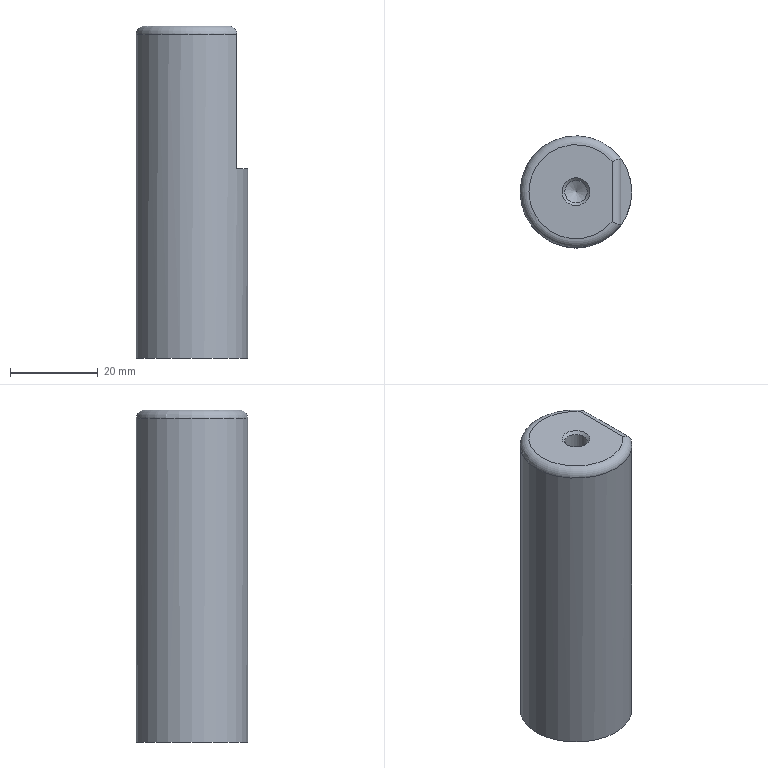Part | STEP file | 1_id1502_x_t | 1 solid | 10 faces | box 25.4 x 25.4 x 75.5 mm | volume 37080 mm3 | plane 4 | cylinder 3 | cone 2 | torus 1 | commonest cylinder face diameters 4 x1 5.105 x1 25.4 x1
STEP:
#1=CARTESIAN_POINT('',(0.,0.,0.));
#2=DIRECTION('',(0.,0.,1.));
#3=DIRECTION('',(1.,0.,0.));
#4=AXIS2_PLACEMENT_3D('',#1,#2,#3);
#5=CARTESIAN_POINT('',(50.2,112.566,-2.));
#6=VERTEX_POINT('',#5);
#7=CARTESIAN_POINT('',(48.2,111.874,0.));
#8=VERTEX_POINT('',#7);
#9=CARTESIAN_POINT('',(50.2,112.566,-2.));
#10=CARTESIAN_POINT('',(50.2,112.566,-1.785));
#11=CARTESIAN_POINT('',(50.164,112.555,-1.566));
#12=CARTESIAN_POINT('',(50.096,112.532,-1.363));
#13=CARTESIAN_POINT('',(50.028,112.509,-1.161));
#14=CARTESIAN_POINT('',(49.926,112.475,-0.9676));
#15=CARTESIAN_POINT('',(49.799,112.433,-0.7989));
#16=CARTESIAN_POINT('',(49.67,112.389,-0.6268));
#17=CARTESIAN_POINT('',(49.512,112.336,-0.4756));
#18=CARTESIAN_POINT('',(49.338,112.276,-0.3554));
#19=CARTESIAN_POINT('',(49.156,112.213,-0.2294));
#20=CARTESIAN_POINT('',(48.952,112.143,-0.134));
#21=CARTESIAN_POINT('',(48.742,112.068,-0.07493));
#22=CARTESIAN_POINT('',(48.569,112.007,-0.02617));
#23=CARTESIAN_POINT('',(48.389,111.943,-0.0009637));
#24=CARTESIAN_POINT('',(48.21,111.878,-0.0000275));
#25=CARTESIAN_POINT('',(48.207,111.876,-0.000009165));
#26=CARTESIAN_POINT('',(48.203,111.875,0.));
#27=CARTESIAN_POINT('',(48.2,111.874,0.));
#28=B_SPLINE_CURVE_WITH_KNOTS('',3,(#9,#10,#11,#12,#13,#14,#15,#16,#17,#18,#19,#20,#21,#22,#23,#24,#25,#26,#27),.UNSPECIFIED.,.F.,.F.,(4,3,3,3,3,3,4),(0.,0.2008,0.4013,0.6058,0.8203,0.9965,1.),.UNSPECIFIED.);
#29=CARTESIAN_POINT('',(40.,105.,-2.));
#30=DIRECTION('',(0.,0.,1.));
#31=DIRECTION('',(1.,0.,0.));
#32=AXIS2_PLACEMENT_3D('',#29,#30,#31);
#33=TOROIDAL_SURFACE('',#32,10.7,2.);
#34=CARTESIAN_POINT('',(0.6382,0.));
#35=CARTESIAN_POINT('',(0.6382,0.01219));
#36=CARTESIAN_POINT('',(0.6383,0.0366));
#37=CARTESIAN_POINT('',(0.6384,0.07331));
#38=CARTESIAN_POINT('',(0.6385,0.1101));
#39=CARTESIAN_POINT('',(0.6388,0.1469));
#40=CARTESIAN_POINT('',(0.6391,0.1836));
#41=CARTESIAN_POINT('',(0.6395,0.2204));
#42=CARTESIAN_POINT('',(0.6399,0.257));
#43=CARTESIAN_POINT('',(0.6405,0.2936));
#44=CARTESIAN_POINT('',(0.641,0.33));
#45=CARTESIAN_POINT('',(0.6417,0.3664));
#46=CARTESIAN_POINT('',(0.6424,0.4028));
#47=CARTESIAN_POINT('',(0.6432,0.4393));
#48=CARTESIAN_POINT('',(0.6441,0.4757));
#49=CARTESIAN_POINT('',(0.645,0.5121));
#50=CARTESIAN_POINT('',(0.646,0.5484));
#51=CARTESIAN_POINT('',(0.647,0.5846));
#52=CARTESIAN_POINT('',(0.6482,0.6207));
#53=CARTESIAN_POINT('',(0.6493,0.6565));
#54=CARTESIAN_POINT('',(0.6506,0.6924));
#55=CARTESIAN_POINT('',(0.6519,0.7283));
#56=CARTESIAN_POINT('',(0.6532,0.7642));
#57=CARTESIAN_POINT('',(0.6546,0.8));
#58=CARTESIAN_POINT('',(0.6561,0.8357));
#59=CARTESIAN_POINT('',(0.6576,0.8714));
#60=CARTESIAN_POINT('',(0.6592,0.907));
#61=CARTESIAN_POINT('',(0.6608,0.9424));
#62=CARTESIAN_POINT('',(0.6625,0.9776));
#63=CARTESIAN_POINT('',(0.6642,1.013));
#64=CARTESIAN_POINT('',(0.666,1.048));
#65=CARTESIAN_POINT('',(0.6678,1.083));
#66=CARTESIAN_POINT('',(0.6697,1.118));
#67=CARTESIAN_POINT('',(0.6716,1.153));
#68=CARTESIAN_POINT('',(0.6736,1.189));
#69=CARTESIAN_POINT('',(0.6756,1.223));
#70=CARTESIAN_POINT('',(0.6776,1.258));
#71=CARTESIAN_POINT('',(0.6797,1.293));
#72=CARTESIAN_POINT('',(0.6818,1.328));
#73=CARTESIAN_POINT('',(0.684,1.363));
#74=CARTESIAN_POINT('',(0.6862,1.397));
#75=CARTESIAN_POINT('',(0.6884,1.432));
#76=CARTESIAN_POINT('',(0.6907,1.467));
#77=CARTESIAN_POINT('',(0.693,1.502));
#78=CARTESIAN_POINT('',(0.6953,1.536));
#79=CARTESIAN_POINT('',(0.6969,1.559));
#80=CARTESIAN_POINT('',(0.6976,1.571));
#81=B_SPLINE_CURVE_WITH_KNOTS('',3,(#34,#35,#36,#37,#38,#39,#40,#41,#42,#43,#44,#45,#46,#47,#48,#49,#50,#51,#52,#53,#54,#55,#56,#57,#58,#59,#60,#61,#62,#63,#64,#65,#66,#67,#68,#69,#70,#71,#72,#73,#74,#75,#76,#77,#78,#79,#80),.UNSPECIFIED.,.F.,.F.,(4,1,1,1,1,1,1,1,1,1,1,1,1,1,1,1,1,1,1,1,1,1,1,1,1,1,1,1,1,1,1,1,1,1,1,1,1,1,1,1,1,1,1,1,4),(0.,0.02273,0.04545,0.06818,0.09091,0.1136,0.1364,0.1591,0.1818,0.2045,0.2273,0.25,0.2727,0.2955,0.3182,0.3409,0.3636,0.3864,0.4091,0.4318,0.4545,0.4773,0.5,0.5227,0.5455,0.5682,0.5909,0.6136,0.6364,0.6591,0.6818,0.7045,0.7273,0.75,0.7727,0.7955,0.8182,0.8409,0.8636,0.8864,0.9091,0.9318,0.9545,0.9773,1.),.QUASI_UNIFORM_KNOTS.);
#82=(GEOMETRIC_REPRESENTATION_CONTEXT(2)PARAMETRIC_REPRESENTATION_CONTEXT()REPRESENTATION_CONTEXT('',''));
#83=DEFINITIONAL_REPRESENTATION('',(#81),#82);
#84=PCURVE('',#33,#83);
#85=CARTESIAN_POINT('',(48.2,105.,-2.));
#86=DIRECTION('',(0.,1.,0.));
#87=DIRECTION('',(0.,0.,1.));
#88=AXIS2_PLACEMENT_3D('',#85,#86,#87);
#89=CYLINDRICAL_SURFACE('',#88,2.);
#90=CARTESIAN_POINT('',(1.571,7.566));
#91=CARTESIAN_POINT('',(1.559,7.566));
#92=CARTESIAN_POINT('',(1.534,7.566));
#93=CARTESIAN_POINT('',(1.497,7.565));
#94=CARTESIAN_POINT('',(1.461,7.562));
#95=CARTESIAN_POINT('',(1.424,7.559));
#96=CARTESIAN_POINT('',(1.387,7.555));
#97=CARTESIAN_POINT('',(1.35,7.55));
#98=CARTESIAN_POINT('',(1.314,7.545));
#99=CARTESIAN_POINT('',(1.277,7.538));
#100=CARTESIAN_POINT('',(1.241,7.531));
#101=CARTESIAN_POINT('',(1.204,7.523));
#102=CARTESIAN_POINT('',(1.168,7.513));
#103=CARTESIAN_POINT('',(1.132,7.503));
#104=CARTESIAN_POINT('',(1.095,7.493));
#105=CARTESIAN_POINT('',(1.059,7.481));
#106=CARTESIAN_POINT('',(1.022,7.469));
#107=CARTESIAN_POINT('',(0.9862,7.456));
#108=CARTESIAN_POINT('',(0.9501,7.442));
#109=CARTESIAN_POINT('',(0.9143,7.428));
#110=CARTESIAN_POINT('',(0.8784,7.413));
#111=CARTESIAN_POINT('',(0.8425,7.397));
#112=CARTESIAN_POINT('',(0.8066,7.38));
#113=CARTESIAN_POINT('',(0.7708,7.363));
#114=CARTESIAN_POINT('',(0.735,7.346));
#115=CARTESIAN_POINT('',(0.6994,7.327));
#116=CARTESIAN_POINT('',(0.6638,7.308));
#117=CARTESIAN_POINT('',(0.6284,7.289));
#118=CARTESIAN_POINT('',(0.5932,7.269));
#119=CARTESIAN_POINT('',(0.558,7.249));
#120=CARTESIAN_POINT('',(0.5228,7.228));
#121=CARTESIAN_POINT('',(0.4876,7.207));
#122=CARTESIAN_POINT('',(0.4524,7.185));
#123=CARTESIAN_POINT('',(0.4173,7.163));
#124=CARTESIAN_POINT('',(0.3823,7.14));
#125=CARTESIAN_POINT('',(0.3473,7.117));
#126=CARTESIAN_POINT('',(0.3125,7.094));
#127=CARTESIAN_POINT('',(0.2778,7.071));
#128=CARTESIAN_POINT('',(0.243,7.047));
#129=CARTESIAN_POINT('',(0.2082,7.023));
#130=CARTESIAN_POINT('',(0.1734,6.998));
#131=CARTESIAN_POINT('',(0.1386,6.974));
#132=CARTESIAN_POINT('',(0.1039,6.949));
#133=CARTESIAN_POINT('',(0.06917,6.924));
#134=CARTESIAN_POINT('',(0.03452,6.899));
#135=CARTESIAN_POINT('',(0.01149,6.882));
#136=CARTESIAN_POINT('',(0.,6.874));
#137=B_SPLINE_CURVE_WITH_KNOTS('',3,(#90,#91,#92,#93,#94,#95,#96,#97,#98,#99,#100,#101,#102,#103,#104,#105,#106,#107,#108,#109,#110,#111,#112,#113,#114,#115,#116,#117,#118,#119,#120,#121,#122,#123,#124,#125,#126,#127,#128,#129,#130,#131,#132,#133,#134,#135,#136),.UNSPECIFIED.,.F.,.F.,(4,1,1,1,1,1,1,1,1,1,1,1,1,1,1,1,1,1,1,1,1,1,1,1,1,1,1,1,1,1,1,1,1,1,1,1,1,1,1,1,1,1,1,1,4),(0.,0.02273,0.04545,0.06818,0.09091,0.1136,0.1364,0.1591,0.1818,0.2045,0.2273,0.25,0.2727,0.2955,0.3182,0.3409,0.3636,0.3864,0.4091,0.4318,0.4545,0.4773,0.5,0.5227,0.5455,0.5682,0.5909,0.6136,0.6364,0.6591,0.6818,0.7045,0.7273,0.75,0.7727,0.7955,0.8182,0.8409,0.8636,0.8864,0.9091,0.9318,0.9545,0.9773,1.),.QUASI_UNIFORM_KNOTS.);
#138=(GEOMETRIC_REPRESENTATION_CONTEXT(2)PARAMETRIC_REPRESENTATION_CONTEXT()REPRESENTATION_CONTEXT('',''));
#139=DEFINITIONAL_REPRESENTATION('',(#137),#138);
#140=PCURVE('',#89,#139);
#141=SURFACE_CURVE('',#28,(#84,#140),.PCURVE_S1.);
#142=EDGE_CURVE('',#6,#8,#141,.T.);
#143=ORIENTED_EDGE('',*,*,#142,.F.);
#144=CARTESIAN_POINT('',(27.3,105.,-2.));
#145=VERTEX_POINT('',#144);
#146=CARTESIAN_POINT('',(40.,105.,-2.));
#147=DIRECTION('',(0.,0.,1.));
#148=DIRECTION('',(-1.,0.,0.));
#149=AXIS2_PLACEMENT_3D('',#146,#147,#148);
#150=CIRCLE('',#149,12.7);
#151=CARTESIAN_POINT('',(-3.142,0.));
#152=DIRECTION('',(1.,0.));
#153=VECTOR('',#152,1.);
#154=LINE('',#151,#153);
#155=(GEOMETRIC_REPRESENTATION_CONTEXT(2)PARAMETRIC_REPRESENTATION_CONTEXT()REPRESENTATION_CONTEXT('',''));
#156=DEFINITIONAL_REPRESENTATION('',(#154),#155);
#157=PCURVE('',#33,#156);
#158=CARTESIAN_POINT('',(40.,105.,0.));
#159=DIRECTION('',(0.,0.,-1.));
#160=DIRECTION('',(-1.,0.,0.));
#161=AXIS2_PLACEMENT_3D('',#158,#159,#160);
#162=CYLINDRICAL_SURFACE('',#161,12.7);
#163=CARTESIAN_POINT('',(6.283,2.));
#164=DIRECTION('',(-1.,0.));
#165=VECTOR('',#164,1.);
#166=LINE('',#163,#165);
#167=(GEOMETRIC_REPRESENTATION_CONTEXT(2)PARAMETRIC_REPRESENTATION_CONTEXT()REPRESENTATION_CONTEXT('',''));
#168=DEFINITIONAL_REPRESENTATION('',(#166),#167);
#169=PCURVE('',#162,#168);
#170=SURFACE_CURVE('',#150,(#157,#169),.PCURVE_S1.);
#171=EDGE_CURVE('',#6,#145,#170,.T.);
#172=ORIENTED_EDGE('',*,*,#171,.T.);
#173=CARTESIAN_POINT('',(50.2,97.434,-2.));
#174=VERTEX_POINT('',#173);
#175=CARTESIAN_POINT('',(40.,105.,-2.));
#176=DIRECTION('',(0.,0.,1.));
#177=DIRECTION('',(-1.,0.,0.));
#178=AXIS2_PLACEMENT_3D('',#175,#176,#177);
#179=CIRCLE('',#178,12.7);
#180=CARTESIAN_POINT('',(-3.142,0.));
#181=DIRECTION('',(1.,0.));
#182=VECTOR('',#181,1.);
#183=LINE('',#180,#182);
#184=(GEOMETRIC_REPRESENTATION_CONTEXT(2)PARAMETRIC_REPRESENTATION_CONTEXT()REPRESENTATION_CONTEXT('',''));
#185=DEFINITIONAL_REPRESENTATION('',(#183),#184);
#186=PCURVE('',#33,#185);
#187=CARTESIAN_POINT('',(12.566,2.));
#188=DIRECTION('',(-1.,0.));
#189=VECTOR('',#188,1.);
#190=LINE('',#187,#189);
#191=(GEOMETRIC_REPRESENTATION_CONTEXT(2)PARAMETRIC_REPRESENTATION_CONTEXT()REPRESENTATION_CONTEXT('',''));
#192=DEFINITIONAL_REPRESENTATION('',(#190),#191);
#193=PCURVE('',#162,#192);
#194=SURFACE_CURVE('',#179,(#186,#193),.PCURVE_S1.);
#195=EDGE_CURVE('',#145,#174,#194,.T.);
#196=ORIENTED_EDGE('',*,*,#195,.T.);
#197=CARTESIAN_POINT('',(48.2,98.126,0.));
#198=VERTEX_POINT('',#197);
#199=CARTESIAN_POINT('',(48.2,98.126,0.));
#200=CARTESIAN_POINT('',(48.203,98.125,0.));
#201=CARTESIAN_POINT('',(48.207,98.124,-0.000009165));
#202=CARTESIAN_POINT('',(48.21,98.122,-0.0000275));
#203=CARTESIAN_POINT('',(48.444,98.038,-0.00125));
#204=CARTESIAN_POINT('',(48.68,97.953,-0.04429));
#205=CARTESIAN_POINT('',(48.901,97.876,-0.1269));
#206=CARTESIAN_POINT('',(49.122,97.798,-0.2096));
#207=CARTESIAN_POINT('',(49.333,97.725,-0.3346));
#208=CARTESIAN_POINT('',(49.515,97.664,-0.4927));
#209=CARTESIAN_POINT('',(49.689,97.604,-0.6451));
#210=CARTESIAN_POINT('',(49.841,97.553,-0.8331));
#211=CARTESIAN_POINT('',(49.955,97.515,-1.041));
#212=CARTESIAN_POINT('',(50.062,97.479,-1.237));
#213=CARTESIAN_POINT('',(50.138,97.454,-1.456));
#214=CARTESIAN_POINT('',(50.174,97.442,-1.679));
#215=CARTESIAN_POINT('',(50.191,97.437,-1.785));
#216=CARTESIAN_POINT('',(50.2,97.434,-1.893));
#217=CARTESIAN_POINT('',(50.2,97.434,-2.));
#218=B_SPLINE_CURVE_WITH_KNOTS('',3,(#199,#200,#201,#202,#203,#204,#205,#206,#207,#208,#209,#210,#211,#212,#213,#214,#215,#216,#217),.UNSPECIFIED.,.F.,.F.,(4,3,3,3,3,3,4),(0.,0.003466,0.2346,0.4662,0.6895,0.9003,1.),.UNSPECIFIED.);
#219=CARTESIAN_POINT('',(5.586,1.571));
#220=CARTESIAN_POINT('',(5.586,1.559));
#221=CARTESIAN_POINT('',(5.588,1.536));
#222=CARTESIAN_POINT('',(5.59,1.502));
#223=CARTESIAN_POINT('',(5.592,1.467));
#224=CARTESIAN_POINT('',(5.595,1.433));
#225=CARTESIAN_POINT('',(5.597,1.398));
#226=CARTESIAN_POINT('',(5.599,1.363));
#227=CARTESIAN_POINT('',(5.601,1.328));
#228=CARTESIAN_POINT('',(5.603,1.293));
#229=CARTESIAN_POINT('',(5.606,1.259));
#230=CARTESIAN_POINT('',(5.608,1.224));
#231=CARTESIAN_POINT('',(5.61,1.189));
#232=CARTESIAN_POINT('',(5.612,1.154));
#233=CARTESIAN_POINT('',(5.613,1.119));
#234=CARTESIAN_POINT('',(5.615,1.084));
#235=CARTESIAN_POINT('',(5.617,1.049));
#236=CARTESIAN_POINT('',(5.619,1.013));
#237=CARTESIAN_POINT('',(5.621,0.978));
#238=CARTESIAN_POINT('',(5.622,0.9426));
#239=CARTESIAN_POINT('',(5.624,0.9072));
#240=CARTESIAN_POINT('',(5.626,0.8718));
#241=CARTESIAN_POINT('',(5.627,0.8364));
#242=CARTESIAN_POINT('',(5.629,0.8008));
#243=CARTESIAN_POINT('',(5.63,0.765));
#244=CARTESIAN_POINT('',(5.631,0.7292));
#245=CARTESIAN_POINT('',(5.633,0.6932));
#246=CARTESIAN_POINT('',(5.634,0.6571));
#247=CARTESIAN_POINT('',(5.635,0.621));
#248=CARTESIAN_POINT('',(5.636,0.5849));
#249=CARTESIAN_POINT('',(5.637,0.5487));
#250=CARTESIAN_POINT('',(5.638,0.5126));
#251=CARTESIAN_POINT('',(5.639,0.4765));
#252=CARTESIAN_POINT('',(5.64,0.4401));
#253=CARTESIAN_POINT('',(5.641,0.4037));
#254=CARTESIAN_POINT('',(5.641,0.3671));
#255=CARTESIAN_POINT('',(5.642,0.3305));
#256=CARTESIAN_POINT('',(5.643,0.2938));
#257=CARTESIAN_POINT('',(5.643,0.2571));
#258=CARTESIAN_POINT('',(5.644,0.2204));
#259=CARTESIAN_POINT('',(5.644,0.1838));
#260=CARTESIAN_POINT('',(5.644,0.1472));
#261=CARTESIAN_POINT('',(5.645,0.1104));
#262=CARTESIAN_POINT('',(5.645,0.0736));
#263=CARTESIAN_POINT('',(5.645,0.03678));
#264=CARTESIAN_POINT('',(5.645,0.01225));
#265=CARTESIAN_POINT('',(5.645,0.));
#266=B_SPLINE_CURVE_WITH_KNOTS('',3,(#219,#220,#221,#222,#223,#224,#225,#226,#227,#228,#229,#230,#231,#232,#233,#234,#235,#236,#237,#238,#239,#240,#241,#242,#243,#244,#245,#246,#247,#248,#249,#250,#251,#252,#253,#254,#255,#256,#257,#258,#259,#260,#261,#262,#263,#264,#265),.UNSPECIFIED.,.F.,.F.,(4,1,1,1,1,1,1,1,1,1,1,1,1,1,1,1,1,1,1,1,1,1,1,1,1,1,1,1,1,1,1,1,1,1,1,1,1,1,1,1,1,1,1,1,4),(0.,0.02273,0.04545,0.06818,0.09091,0.1136,0.1364,0.1591,0.1818,0.2045,0.2273,0.25,0.2727,0.2955,0.3182,0.3409,0.3636,0.3864,0.4091,0.4318,0.4545,0.4773,0.5,0.5227,0.5455,0.5682,0.5909,0.6136,0.6364,0.6591,0.6818,0.7045,0.7273,0.75,0.7727,0.7955,0.8182,0.8409,0.8636,0.8864,0.9091,0.9318,0.9545,0.9773,1.),.QUASI_UNIFORM_KNOTS.);
#267=(GEOMETRIC_REPRESENTATION_CONTEXT(2)PARAMETRIC_REPRESENTATION_CONTEXT()REPRESENTATION_CONTEXT('',''));
#268=DEFINITIONAL_REPRESENTATION('',(#266),#267);
#269=PCURVE('',#33,#268);
#270=CARTESIAN_POINT('',(0.,-6.874));
#271=CARTESIAN_POINT('',(0.01146,-6.882));
#272=CARTESIAN_POINT('',(0.03441,-6.899));
#273=CARTESIAN_POINT('',(0.06894,-6.924));
#274=CARTESIAN_POINT('',(0.1036,-6.949));
#275=CARTESIAN_POINT('',(0.1382,-6.973));
#276=CARTESIAN_POINT('',(0.173,-6.998));
#277=CARTESIAN_POINT('',(0.2078,-7.022));
#278=CARTESIAN_POINT('',(0.2426,-7.046));
#279=CARTESIAN_POINT('',(0.2774,-7.07));
#280=CARTESIAN_POINT('',(0.3122,-7.094));
#281=CARTESIAN_POINT('',(0.347,-7.117));
#282=CARTESIAN_POINT('',(0.3817,-7.14));
#283=CARTESIAN_POINT('',(0.4166,-7.162));
#284=CARTESIAN_POINT('',(0.4517,-7.184));
#285=CARTESIAN_POINT('',(0.4868,-7.206));
#286=CARTESIAN_POINT('',(0.5221,-7.228));
#287=CARTESIAN_POINT('',(0.5574,-7.248));
#288=CARTESIAN_POINT('',(0.5928,-7.269));
#289=CARTESIAN_POINT('',(0.6282,-7.289));
#290=CARTESIAN_POINT('',(0.6636,-7.308));
#291=CARTESIAN_POINT('',(0.699,-7.327));
#292=CARTESIAN_POINT('',(0.7344,-7.345));
#293=CARTESIAN_POINT('',(0.77,-7.363));
#294=CARTESIAN_POINT('',(0.8058,-7.38));
#295=CARTESIAN_POINT('',(0.8416,-7.397));
#296=CARTESIAN_POINT('',(0.8776,-7.412));
#297=CARTESIAN_POINT('',(0.9137,-7.428));
#298=CARTESIAN_POINT('',(0.9498,-7.442));
#299=CARTESIAN_POINT('',(0.9859,-7.456));
#300=CARTESIAN_POINT('',(1.022,-7.469));
#301=CARTESIAN_POINT('',(1.058,-7.481));
#302=CARTESIAN_POINT('',(1.094,-7.493));
#303=CARTESIAN_POINT('',(1.131,-7.503));
#304=CARTESIAN_POINT('',(1.167,-7.513));
#305=CARTESIAN_POINT('',(1.204,-7.522));
#306=CARTESIAN_POINT('',(1.24,-7.531));
#307=CARTESIAN_POINT('',(1.277,-7.538));
#308=CARTESIAN_POINT('',(1.314,-7.545));
#309=CARTESIAN_POINT('',(1.35,-7.55));
#310=CARTESIAN_POINT('',(1.387,-7.555));
#311=CARTESIAN_POINT('',(1.424,-7.559));
#312=CARTESIAN_POINT('',(1.46,-7.562));
#313=CARTESIAN_POINT('',(1.497,-7.565));
#314=CARTESIAN_POINT('',(1.534,-7.566));
#315=CARTESIAN_POINT('',(1.559,-7.566));
#316=CARTESIAN_POINT('',(1.571,-7.566));
#317=B_SPLINE_CURVE_WITH_KNOTS('',3,(#270,#271,#272,#273,#274,#275,#276,#277,#278,#279,#280,#281,#282,#283,#284,#285,#286,#287,#288,#289,#290,#291,#292,#293,#294,#295,#296,#297,#298,#299,#300,#301,#302,#303,#304,#305,#306,#307,#308,#309,#310,#311,#312,#313,#314,#315,#316),.UNSPECIFIED.,.F.,.F.,(4,1,1,1,1,1,1,1,1,1,1,1,1,1,1,1,1,1,1,1,1,1,1,1,1,1,1,1,1,1,1,1,1,1,1,1,1,1,1,1,1,1,1,1,4),(0.,0.02273,0.04545,0.06818,0.09091,0.1136,0.1364,0.1591,0.1818,0.2045,0.2273,0.25,0.2727,0.2955,0.3182,0.3409,0.3636,0.3864,0.4091,0.4318,0.4545,0.4773,0.5,0.5227,0.5455,0.5682,0.5909,0.6136,0.6364,0.6591,0.6818,0.7045,0.7273,0.75,0.7727,0.7955,0.8182,0.8409,0.8636,0.8864,0.9091,0.9318,0.9545,0.9773,1.),.QUASI_UNIFORM_KNOTS.);
#318=(GEOMETRIC_REPRESENTATION_CONTEXT(2)PARAMETRIC_REPRESENTATION_CONTEXT()REPRESENTATION_CONTEXT('',''));
#319=DEFINITIONAL_REPRESENTATION('',(#317),#318);
#320=PCURVE('',#89,#319);
#321=SURFACE_CURVE('',#218,(#269,#320),.PCURVE_S1.);
#322=EDGE_CURVE('',#198,#174,#321,.T.);
#323=ORIENTED_EDGE('',*,*,#322,.F.);
#324=CARTESIAN_POINT('',(40.,105.,0.));
#325=DIRECTION('',(0.,0.,1.));
#326=DIRECTION('',(0.7664,0.6424,0.));
#327=AXIS2_PLACEMENT_3D('',#324,#325,#326);
#328=CIRCLE('',#327,10.7);
#329=CARTESIAN_POINT('',(0.6976,1.571));
#330=DIRECTION('',(1.,0.));
#331=VECTOR('',#330,1.);
#332=LINE('',#329,#331);
#333=(GEOMETRIC_REPRESENTATION_CONTEXT(2)PARAMETRIC_REPRESENTATION_CONTEXT()REPRESENTATION_CONTEXT('',''));
#334=DEFINITIONAL_REPRESENTATION('',(#332),#333);
#335=PCURVE('',#33,#334);
#336=CARTESIAN_POINT('',(40.,105.,0.));
#337=DIRECTION('',(0.,0.,1.));
#338=DIRECTION('',(1.,0.,0.));
#339=AXIS2_PLACEMENT_3D('',#336,#337,#338);
#340=PLANE('',#339);
#341=CARTESIAN_POINT('',(0.,0.));
#342=DIRECTION('',(0.7664,0.6424));
#343=AXIS2_PLACEMENT_2D('',#341,#342);
#344=CIRCLE('',#343,10.7);
#345=(GEOMETRIC_REPRESENTATION_CONTEXT(2)PARAMETRIC_REPRESENTATION_CONTEXT()REPRESENTATION_CONTEXT('',''));
#346=DEFINITIONAL_REPRESENTATION('',(#344),#345);
#347=PCURVE('',#340,#346);
#348=SURFACE_CURVE('',#328,(#335,#347),.PCURVE_S1.);
#349=EDGE_CURVE('',#8,#198,#348,.T.);
#350=ORIENTED_EDGE('',*,*,#349,.F.);
#351=EDGE_LOOP('',(#143,#172,#196,#323,#350));
#352=FACE_BOUND('',#351,.T.);
#353=ADVANCED_FACE('',(#352),#33,.T.);
#354=ORIENTED_EDGE('',*,*,#349,.T.);
#355=CARTESIAN_POINT('',(48.2,111.874,0.));
#356=DIRECTION('',(0.,-1.,0.));
#357=VECTOR('',#356,1.);
#358=LINE('',#355,#357);
#359=CARTESIAN_POINT('',(8.2,6.874));
#360=DIRECTION('',(0.,-1.));
#361=VECTOR('',#360,1.);
#362=LINE('',#359,#361);
#363=(GEOMETRIC_REPRESENTATION_CONTEXT(2)PARAMETRIC_REPRESENTATION_CONTEXT()REPRESENTATION_CONTEXT('',''));
#364=DEFINITIONAL_REPRESENTATION('',(#362),#363);
#365=PCURVE('',#340,#364);
#366=CARTESIAN_POINT('',(0.,6.874));
#367=DIRECTION('',(0.,-1.));
#368=VECTOR('',#367,1.);
#369=LINE('',#366,#368);
#370=(GEOMETRIC_REPRESENTATION_CONTEXT(2)PARAMETRIC_REPRESENTATION_CONTEXT()REPRESENTATION_CONTEXT('',''));
#371=DEFINITIONAL_REPRESENTATION('',(#369),#370);
#372=PCURVE('',#89,#371);
#373=SURFACE_CURVE('',#358,(#365,#372),.PCURVE_S1.);
#374=EDGE_CURVE('',#8,#198,#373,.T.);
#375=ORIENTED_EDGE('',*,*,#374,.F.);
#376=EDGE_LOOP('',(#354,#375));
#377=FACE_BOUND('',#376,.T.);
#378=CARTESIAN_POINT('',(36.825,105.,0.));
#379=VERTEX_POINT('',#378);
#380=CARTESIAN_POINT('',(40.,105.,0.));
#381=DIRECTION('',(0.,0.,-1.));
#382=DIRECTION('',(-1.,0.,0.));
#383=AXIS2_PLACEMENT_3D('',#380,#381,#382);
#384=CIRCLE('',#383,3.175);
#385=CARTESIAN_POINT('',(-3.175,0.));
#386=CARTESIAN_POINT('',(-3.175,5.499));
#387=CARTESIAN_POINT('',(1.588,2.75));
#388=CARTESIAN_POINT('',(6.35,0.));
#389=CARTESIAN_POINT('',(1.588,-2.75));
#390=CARTESIAN_POINT('',(-3.175,-5.499));
#391=CARTESIAN_POINT('',(-3.175,0.));
#392=(BOUNDED_CURVE()B_SPLINE_CURVE(2,(#385,#386,#387,#388,#389,#390,#391),.UNSPECIFIED.,.T.,.F.)B_SPLINE_CURVE_WITH_KNOTS((1,2,2,2,2,1),(-2.094,0.,2.094,4.189,6.283,8.378),.UNSPECIFIED.)CURVE()GEOMETRIC_REPRESENTATION_ITEM()RATIONAL_B_SPLINE_CURVE((1.,0.5,1.,0.5,1.,0.5,1.))REPRESENTATION_ITEM(''));
#393=(GEOMETRIC_REPRESENTATION_CONTEXT(2)PARAMETRIC_REPRESENTATION_CONTEXT()REPRESENTATION_CONTEXT('',''));
#394=DEFINITIONAL_REPRESENTATION('',(#392),#393);
#395=PCURVE('',#340,#394);
#396=CARTESIAN_POINT('',(40.,105.,-0.3112));
#397=DIRECTION('',(0.,0.,1.));
#398=DIRECTION('',(1.,0.,0.));
#399=AXIS2_PLACEMENT_3D('',#396,#397,#398);
#400=CONICAL_SURFACE('',#399,2.864,0.7854);
#401=CARTESIAN_POINT('',(9.425,0.3112));
#402=DIRECTION('',(-1.,0.));
#403=VECTOR('',#402,1.);
#404=LINE('',#401,#403);
#405=(GEOMETRIC_REPRESENTATION_CONTEXT(2)PARAMETRIC_REPRESENTATION_CONTEXT()REPRESENTATION_CONTEXT('',''));
#406=DEFINITIONAL_REPRESENTATION('',(#404),#405);
#407=PCURVE('',#400,#406);
#408=SURFACE_CURVE('',#384,(#395,#407),.PCURVE_S1.);
#409=EDGE_CURVE('',#379,#379,#408,.T.);
#410=ORIENTED_EDGE('',*,*,#409,.T.);
#411=EDGE_LOOP('',(#410));
#412=FACE_BOUND('',#411,.T.);
#413=ADVANCED_FACE('',(#377,#412),#340,.T.);
#414=ORIENTED_EDGE('',*,*,#409,.T.);
#415=CARTESIAN_POINT('',(37.447,105.,-0.6223));
#416=VERTEX_POINT('',#415);
#417=CARTESIAN_POINT('',(37.447,105.,-0.6223));
#418=CARTESIAN_POINT('',(36.825,105.,0.));
#419=B_SPLINE_CURVE_WITH_KNOTS('',1,(#417,#418),.UNSPECIFIED.,.F.,.F.,(2,2),(-0.44,0.44),.PIECEWISE_BEZIER_KNOTS.);
#420=CARTESIAN_POINT('',(3.142,0.));
#421=DIRECTION('',(0.,1.));
#422=VECTOR('',#421,1.);
#423=LINE('',#420,#422);
#424=(GEOMETRIC_REPRESENTATION_CONTEXT(2)PARAMETRIC_REPRESENTATION_CONTEXT()REPRESENTATION_CONTEXT('',''));
#425=DEFINITIONAL_REPRESENTATION('',(#423),#424);
#426=PCURVE('',#400,#425);
#427=CARTESIAN_POINT('',(9.425,0.));
#428=DIRECTION('',(0.,1.));
#429=VECTOR('',#428,1.);
#430=LINE('',#427,#429);
#431=(GEOMETRIC_REPRESENTATION_CONTEXT(2)PARAMETRIC_REPRESENTATION_CONTEXT()REPRESENTATION_CONTEXT('',''));
#432=DEFINITIONAL_REPRESENTATION('',(#430),#431);
#433=PCURVE('',#400,#432);
#434=SEAM_CURVE('',#419,(#426,#433),.PCURVE_S1.);
#435=EDGE_CURVE('',#416,#379,#434,.T.);
#436=ORIENTED_EDGE('',*,*,#435,.F.);
#437=CARTESIAN_POINT('',(40.,105.,-0.6223));
#438=DIRECTION('',(0.,0.,-1.));
#439=DIRECTION('',(-1.,0.,0.));
#440=AXIS2_PLACEMENT_3D('',#437,#438,#439);
#441=CIRCLE('',#440,2.553);
#442=CARTESIAN_POINT('',(9.425,-0.3112));
#443=DIRECTION('',(-1.,0.));
#444=VECTOR('',#443,1.);
#445=LINE('',#442,#444);
#446=(GEOMETRIC_REPRESENTATION_CONTEXT(2)PARAMETRIC_REPRESENTATION_CONTEXT()REPRESENTATION_CONTEXT('',''));
#447=DEFINITIONAL_REPRESENTATION('',(#445),#446);
#448=PCURVE('',#400,#447);
#449=CARTESIAN_POINT('',(40.,105.,0.));
#450=DIRECTION('',(0.,0.,-1.));
#451=DIRECTION('',(-1.,0.,0.));
#452=AXIS2_PLACEMENT_3D('',#449,#450,#451);
#453=CYLINDRICAL_SURFACE('',#452,2.553);
#454=CARTESIAN_POINT('',(0.,0.6223));
#455=DIRECTION('',(1.,0.));
#456=VECTOR('',#455,1.);
#457=LINE('',#454,#456);
#458=(GEOMETRIC_REPRESENTATION_CONTEXT(2)PARAMETRIC_REPRESENTATION_CONTEXT()REPRESENTATION_CONTEXT('',''));
#459=DEFINITIONAL_REPRESENTATION('',(#457),#458);
#460=PCURVE('',#453,#459);
#461=SURFACE_CURVE('',#441,(#448,#460),.PCURVE_S1.);
#462=EDGE_CURVE('',#416,#416,#461,.T.);
#463=ORIENTED_EDGE('',*,*,#462,.F.);
#464=ORIENTED_EDGE('',*,*,#435,.T.);
#465=EDGE_LOOP('',(#414,#436,#463,#464));
#466=FACE_BOUND('',#465,.F.);
#467=ADVANCED_FACE('',(#466),#400,.F.);
#468=CARTESIAN_POINT('',(42.553,105.,-12.7));
#469=VERTEX_POINT('',#468);
#470=CARTESIAN_POINT('',(37.447,105.,-12.7));
#471=VERTEX_POINT('',#470);
#472=CARTESIAN_POINT('',(40.,105.,-12.7));
#473=DIRECTION('',(0.,0.,1.));
#474=DIRECTION('',(1.,0.,0.));
#475=AXIS2_PLACEMENT_3D('',#472,#473,#474);
#476=CIRCLE('',#475,2.553);
#477=CARTESIAN_POINT('',(3.142,12.7));
#478=DIRECTION('',(-1.,0.));
#479=VECTOR('',#478,1.);
#480=LINE('',#477,#479);
#481=(GEOMETRIC_REPRESENTATION_CONTEXT(2)PARAMETRIC_REPRESENTATION_CONTEXT()REPRESENTATION_CONTEXT('',''));
#482=DEFINITIONAL_REPRESENTATION('',(#480),#481);
#483=PCURVE('',#453,#482);
#484=CARTESIAN_POINT('',(40.,105.,-13.441));
#485=DIRECTION('',(0.,0.,1.));
#486=DIRECTION('',(1.,0.,0.));
#487=AXIS2_PLACEMENT_3D('',#484,#485,#486);
#488=CONICAL_SURFACE('',#487,1.319,1.03);
#489=CARTESIAN_POINT('',(0.,0.7411));
#490=DIRECTION('',(1.,0.));
#491=VECTOR('',#490,1.);
#492=LINE('',#489,#491);
#493=(GEOMETRIC_REPRESENTATION_CONTEXT(2)PARAMETRIC_REPRESENTATION_CONTEXT()REPRESENTATION_CONTEXT('',''));
#494=DEFINITIONAL_REPRESENTATION('',(#492),#493);
#495=PCURVE('',#488,#494);
#496=SURFACE_CURVE('',#476,(#483,#495),.PCURVE_S1.);
#497=EDGE_CURVE('',#469,#471,#496,.T.);
#498=ORIENTED_EDGE('',*,*,#497,.T.);
#499=CARTESIAN_POINT('',(37.447,105.,-0.6223));
#500=CARTESIAN_POINT('',(37.447,105.,-12.7));
#501=B_SPLINE_CURVE_WITH_KNOTS('',1,(#499,#500),.UNSPECIFIED.,.F.,.F.,(2,2),(0.6223,12.7),.PIECEWISE_BEZIER_KNOTS.);
#502=CARTESIAN_POINT('',(0.,0.));
#503=DIRECTION('',(0.,1.));
#504=VECTOR('',#503,1.);
#505=LINE('',#502,#504);
#506=(GEOMETRIC_REPRESENTATION_CONTEXT(2)PARAMETRIC_REPRESENTATION_CONTEXT()REPRESENTATION_CONTEXT('',''));
#507=DEFINITIONAL_REPRESENTATION('',(#505),#506);
#508=PCURVE('',#453,#507);
#509=CARTESIAN_POINT('',(6.283,0.));
#510=DIRECTION('',(0.,1.));
#511=VECTOR('',#510,1.);
#512=LINE('',#509,#511);
#513=(GEOMETRIC_REPRESENTATION_CONTEXT(2)PARAMETRIC_REPRESENTATION_CONTEXT()REPRESENTATION_CONTEXT('',''));
#514=DEFINITIONAL_REPRESENTATION('',(#512),#513);
#515=PCURVE('',#453,#514);
#516=SEAM_CURVE('',#501,(#508,#515),.PCURVE_S1.);
#517=EDGE_CURVE('',#416,#471,#516,.T.);
#518=ORIENTED_EDGE('',*,*,#517,.F.);
#519=ORIENTED_EDGE('',*,*,#462,.T.);
#520=ORIENTED_EDGE('',*,*,#517,.T.);
#521=CARTESIAN_POINT('',(40.,105.,-12.7));
#522=DIRECTION('',(0.,0.,1.));
#523=DIRECTION('',(1.,0.,0.));
#524=AXIS2_PLACEMENT_3D('',#521,#522,#523);
#525=CIRCLE('',#524,2.553);
#526=CARTESIAN_POINT('',(9.425,12.7));
#527=DIRECTION('',(-1.,0.));
#528=VECTOR('',#527,1.);
#529=LINE('',#526,#528);
#530=(GEOMETRIC_REPRESENTATION_CONTEXT(2)PARAMETRIC_REPRESENTATION_CONTEXT()REPRESENTATION_CONTEXT('',''));
#531=DEFINITIONAL_REPRESENTATION('',(#529),#530);
#532=PCURVE('',#453,#531);
#533=CARTESIAN_POINT('',(0.,0.7411));
#534=DIRECTION('',(1.,0.));
#535=VECTOR('',#534,1.);
#536=LINE('',#533,#535);
#537=(GEOMETRIC_REPRESENTATION_CONTEXT(2)PARAMETRIC_REPRESENTATION_CONTEXT()REPRESENTATION_CONTEXT('',''));
#538=DEFINITIONAL_REPRESENTATION('',(#536),#537);
#539=PCURVE('',#488,#538);
#540=SURFACE_CURVE('',#525,(#532,#539),.PCURVE_S1.);
#541=EDGE_CURVE('',#471,#469,#540,.T.);
#542=ORIENTED_EDGE('',*,*,#541,.T.);
#543=EDGE_LOOP('',(#498,#518,#519,#520,#542));
#544=FACE_BOUND('',#543,.F.);
#545=ADVANCED_FACE('',(#544),#453,.F.);
#546=ORIENTED_EDGE('',*,*,#541,.F.);
#547=ORIENTED_EDGE('',*,*,#497,.F.);
#548=CARTESIAN_POINT('',(40.,105.,-14.234));
#549=VERTEX_POINT('',#548);
#550=CARTESIAN_POINT('',(40.,105.,-14.234));
#551=CARTESIAN_POINT('',(42.553,105.,-12.7));
#552=B_SPLINE_CURVE_WITH_KNOTS('',1,(#550,#551),.UNSPECIFIED.,.F.,.F.,(2,2),(-1.539,1.439),.PIECEWISE_BEZIER_KNOTS.);
#553=CARTESIAN_POINT('',(0.,0.));
#554=DIRECTION('',(0.,1.));
#555=VECTOR('',#554,1.);
#556=LINE('',#553,#555);
#557=(GEOMETRIC_REPRESENTATION_CONTEXT(2)PARAMETRIC_REPRESENTATION_CONTEXT()REPRESENTATION_CONTEXT('',''));
#558=DEFINITIONAL_REPRESENTATION('',(#556),#557);
#559=PCURVE('',#488,#558);
#560=CARTESIAN_POINT('',(6.283,0.));
#561=DIRECTION('',(0.,1.));
#562=VECTOR('',#561,1.);
#563=LINE('',#560,#562);
#564=(GEOMETRIC_REPRESENTATION_CONTEXT(2)PARAMETRIC_REPRESENTATION_CONTEXT()REPRESENTATION_CONTEXT('',''));
#565=DEFINITIONAL_REPRESENTATION('',(#563),#564);
#566=PCURVE('',#488,#565);
#567=SEAM_CURVE('',#552,(#559,#566),.PCURVE_S1.);
#568=EDGE_CURVE('',#549,#469,#567,.T.);
#569=ORIENTED_EDGE('',*,*,#568,.F.);
#570=ORIENTED_EDGE('',*,*,#568,.T.);
#571=EDGE_LOOP('',(#546,#547,#569,#570));
#572=FACE_BOUND('',#571,.F.);
#573=ADVANCED_FACE('',(#572),#488,.F.);
#574=CARTESIAN_POINT('',(50.2,97.434,-2.));
#575=DIRECTION('',(0.,1.,0.));
#576=VECTOR('',#575,1.);
#577=LINE('',#574,#576);
#578=CARTESIAN_POINT('',(1.571,-7.566));
#579=DIRECTION('',(0.,1.));
#580=VECTOR('',#579,1.);
#581=LINE('',#578,#580);
#582=(GEOMETRIC_REPRESENTATION_CONTEXT(2)PARAMETRIC_REPRESENTATION_CONTEXT()REPRESENTATION_CONTEXT('',''));
#583=DEFINITIONAL_REPRESENTATION('',(#581),#582);
#584=PCURVE('',#89,#583);
#585=CARTESIAN_POINT('',(50.2,105.,-24.6));
#586=DIRECTION('',(-1.,0.,0.));
#587=DIRECTION('',(0.,0.,1.));
#588=AXIS2_PLACEMENT_3D('',#585,#586,#587);
#589=PLANE('',#588);
#590=CARTESIAN_POINT('',(22.6,-7.566));
#591=DIRECTION('',(0.,1.));
#592=VECTOR('',#591,1.);
#593=LINE('',#590,#592);
#594=(GEOMETRIC_REPRESENTATION_CONTEXT(2)PARAMETRIC_REPRESENTATION_CONTEXT()REPRESENTATION_CONTEXT('',''));
#595=DEFINITIONAL_REPRESENTATION('',(#593),#594);
#596=PCURVE('',#589,#595);
#597=SURFACE_CURVE('',#577,(#584,#596),.PCURVE_S1.);
#598=EDGE_CURVE('',#174,#6,#597,.T.);
#599=ORIENTED_EDGE('',*,*,#598,.T.);
#600=ORIENTED_EDGE('',*,*,#142,.T.);
#601=ORIENTED_EDGE('',*,*,#374,.T.);
#602=ORIENTED_EDGE('',*,*,#322,.T.);
#603=EDGE_LOOP('',(#599,#600,#601,#602));
#604=FACE_BOUND('',#603,.T.);
#605=ADVANCED_FACE('',(#604),#89,.T.);
#606=ORIENTED_EDGE('',*,*,#598,.F.);
#607=CARTESIAN_POINT('',(50.2,97.434,-32.5));
#608=VERTEX_POINT('',#607);
#609=CARTESIAN_POINT('',(50.2,97.434,-32.5));
#610=DIRECTION('',(0.,0.,1.));
#611=VECTOR('',#610,1.);
#612=LINE('',#609,#611);
#613=CARTESIAN_POINT('',(-7.9,-7.566));
#614=DIRECTION('',(1.,0.));
#615=VECTOR('',#614,1.);
#616=LINE('',#613,#615);
#617=(GEOMETRIC_REPRESENTATION_CONTEXT(2)PARAMETRIC_REPRESENTATION_CONTEXT()REPRESENTATION_CONTEXT('',''));
#618=DEFINITIONAL_REPRESENTATION('',(#616),#617);
#619=PCURVE('',#589,#618);
#620=CARTESIAN_POINT('',(3.78,32.5));
#621=DIRECTION('',(0.,-1.));
#622=VECTOR('',#621,1.);
#623=LINE('',#620,#622);
#624=(GEOMETRIC_REPRESENTATION_CONTEXT(2)PARAMETRIC_REPRESENTATION_CONTEXT()REPRESENTATION_CONTEXT('',''));
#625=DEFINITIONAL_REPRESENTATION('',(#623),#624);
#626=PCURVE('',#162,#625);
#627=SURFACE_CURVE('',#612,(#619,#626),.PCURVE_S1.);
#628=EDGE_CURVE('',#608,#174,#627,.T.);
#629=ORIENTED_EDGE('',*,*,#628,.F.);
#630=CARTESIAN_POINT('',(50.2,112.566,-32.5));
#631=VERTEX_POINT('',#630);
#632=CARTESIAN_POINT('',(50.2,97.434,-32.5));
#633=DIRECTION('',(0.,1.,0.));
#634=VECTOR('',#633,1.);
#635=LINE('',#632,#634);
#636=CARTESIAN_POINT('',(-7.9,-7.566));
#637=DIRECTION('',(0.,1.));
#638=VECTOR('',#637,1.);
#639=LINE('',#636,#638);
#640=(GEOMETRIC_REPRESENTATION_CONTEXT(2)PARAMETRIC_REPRESENTATION_CONTEXT()REPRESENTATION_CONTEXT('',''));
#641=DEFINITIONAL_REPRESENTATION('',(#639),#640);
#642=PCURVE('',#589,#641);
#643=CARTESIAN_POINT('',(52.66,225.874,-32.5));
#644=DIRECTION('',(0.,0.,1.));
#645=DIRECTION('',(1.,0.,0.));
#646=AXIS2_PLACEMENT_3D('',#643,#644,#645);
#647=PLANE('',#646);
#648=CARTESIAN_POINT('',(-2.46,-128.44));
#649=DIRECTION('',(0.,1.));
#650=VECTOR('',#649,1.);
#651=LINE('',#648,#650);
#652=(GEOMETRIC_REPRESENTATION_CONTEXT(2)PARAMETRIC_REPRESENTATION_CONTEXT()REPRESENTATION_CONTEXT('',''));
#653=DEFINITIONAL_REPRESENTATION('',(#651),#652);
#654=PCURVE('',#647,#653);
#655=SURFACE_CURVE('',#635,(#642,#654),.PCURVE_S1.);
#656=EDGE_CURVE('',#608,#631,#655,.T.);
#657=ORIENTED_EDGE('',*,*,#656,.T.);
#658=CARTESIAN_POINT('',(50.2,112.566,-2.));
#659=DIRECTION('',(0.,0.,-1.));
#660=VECTOR('',#659,1.);
#661=LINE('',#658,#660);
#662=CARTESIAN_POINT('',(22.6,7.566));
#663=DIRECTION('',(-1.,0.));
#664=VECTOR('',#663,1.);
#665=LINE('',#662,#664);
#666=(GEOMETRIC_REPRESENTATION_CONTEXT(2)PARAMETRIC_REPRESENTATION_CONTEXT()REPRESENTATION_CONTEXT('',''));
#667=DEFINITIONAL_REPRESENTATION('',(#665),#666);
#668=PCURVE('',#589,#667);
#669=CARTESIAN_POINT('',(2.503,2.));
#670=DIRECTION('',(0.,1.));
#671=VECTOR('',#670,1.);
#672=LINE('',#669,#671);
#673=(GEOMETRIC_REPRESENTATION_CONTEXT(2)PARAMETRIC_REPRESENTATION_CONTEXT()REPRESENTATION_CONTEXT('',''));
#674=DEFINITIONAL_REPRESENTATION('',(#672),#673);
#675=PCURVE('',#162,#674);
#676=SURFACE_CURVE('',#661,(#668,#675),.PCURVE_S1.);
#677=EDGE_CURVE('',#6,#631,#676,.T.);
#678=ORIENTED_EDGE('',*,*,#677,.F.);
#679=EDGE_LOOP('',(#606,#629,#657,#678));
#680=FACE_BOUND('',#679,.T.);
#681=ADVANCED_FACE('',(#680),#589,.F.);
#682=CARTESIAN_POINT('',(27.3,105.,-75.5));
#683=VERTEX_POINT('',#682);
#684=CARTESIAN_POINT('',(40.,105.,-75.5));
#685=DIRECTION('',(0.,0.,-1.));
#686=DIRECTION('',(-1.,0.,0.));
#687=AXIS2_PLACEMENT_3D('',#684,#685,#686);
#688=CIRCLE('',#687,12.7);
#689=CARTESIAN_POINT('',(0.,75.5));
#690=DIRECTION('',(1.,0.));
#691=VECTOR('',#690,1.);
#692=LINE('',#689,#691);
#693=(GEOMETRIC_REPRESENTATION_CONTEXT(2)PARAMETRIC_REPRESENTATION_CONTEXT()REPRESENTATION_CONTEXT('',''));
#694=DEFINITIONAL_REPRESENTATION('',(#692),#693);
#695=PCURVE('',#162,#694);
#696=CARTESIAN_POINT('',(40.,105.,-75.5));
#697=DIRECTION('',(0.,0.,1.));
#698=DIRECTION('',(1.,0.,0.));
#699=AXIS2_PLACEMENT_3D('',#696,#697,#698);
#700=PLANE('',#699);
#701=CARTESIAN_POINT('',(-12.7,0.));
#702=CARTESIAN_POINT('',(-12.7,21.997));
#703=CARTESIAN_POINT('',(6.35,10.999));
#704=CARTESIAN_POINT('',(25.4,0.));
#705=CARTESIAN_POINT('',(6.35,-10.999));
#706=CARTESIAN_POINT('',(-12.7,-21.997));
#707=CARTESIAN_POINT('',(-12.7,0.));
#708=(BOUNDED_CURVE()B_SPLINE_CURVE(2,(#701,#702,#703,#704,#705,#706,#707),.UNSPECIFIED.,.T.,.F.)B_SPLINE_CURVE_WITH_KNOTS((1,2,2,2,2,1),(-2.094,0.,2.094,4.189,6.283,8.378),.UNSPECIFIED.)CURVE()GEOMETRIC_REPRESENTATION_ITEM()RATIONAL_B_SPLINE_CURVE((1.,0.5,1.,0.5,1.,0.5,1.))REPRESENTATION_ITEM(''));
#709=(GEOMETRIC_REPRESENTATION_CONTEXT(2)PARAMETRIC_REPRESENTATION_CONTEXT()REPRESENTATION_CONTEXT('',''));
#710=DEFINITIONAL_REPRESENTATION('',(#708),#709);
#711=PCURVE('',#700,#710);
#712=SURFACE_CURVE('',#688,(#695,#711),.PCURVE_S1.);
#713=EDGE_CURVE('',#683,#683,#712,.T.);
#714=ORIENTED_EDGE('',*,*,#713,.F.);
#715=CARTESIAN_POINT('',(27.3,105.,-2.));
#716=CARTESIAN_POINT('',(27.3,105.,-75.5));
#717=B_SPLINE_CURVE_WITH_KNOTS('',1,(#715,#716),.UNSPECIFIED.,.F.,.F.,(2,2),(2.,75.5),.PIECEWISE_BEZIER_KNOTS.);
#718=CARTESIAN_POINT('',(0.,0.));
#719=DIRECTION('',(0.,1.));
#720=VECTOR('',#719,1.);
#721=LINE('',#718,#720);
#722=(GEOMETRIC_REPRESENTATION_CONTEXT(2)PARAMETRIC_REPRESENTATION_CONTEXT()REPRESENTATION_CONTEXT('',''));
#723=DEFINITIONAL_REPRESENTATION('',(#721),#722);
#724=PCURVE('',#162,#723);
#725=CARTESIAN_POINT('',(6.283,0.));
#726=DIRECTION('',(0.,1.));
#727=VECTOR('',#726,1.);
#728=LINE('',#725,#727);
#729=(GEOMETRIC_REPRESENTATION_CONTEXT(2)PARAMETRIC_REPRESENTATION_CONTEXT()REPRESENTATION_CONTEXT('',''));
#730=DEFINITIONAL_REPRESENTATION('',(#728),#729);
#731=PCURVE('',#162,#730);
#732=SEAM_CURVE('',#717,(#724,#731),.PCURVE_S1.);
#733=EDGE_CURVE('',#145,#683,#732,.T.);
#734=ORIENTED_EDGE('',*,*,#733,.F.);
#735=ORIENTED_EDGE('',*,*,#171,.F.);
#736=ORIENTED_EDGE('',*,*,#677,.T.);
#737=CARTESIAN_POINT('',(40.,105.,-32.5));
#738=DIRECTION('',(0.,0.,1.));
#739=DIRECTION('',(1.,0.,0.));
#740=AXIS2_PLACEMENT_3D('',#737,#738,#739);
#741=CIRCLE('',#740,12.7);
#742=CARTESIAN_POINT('',(9.425,32.5));
#743=DIRECTION('',(-1.,0.));
#744=VECTOR('',#743,1.);
#745=LINE('',#742,#744);
#746=(GEOMETRIC_REPRESENTATION_CONTEXT(2)PARAMETRIC_REPRESENTATION_CONTEXT()REPRESENTATION_CONTEXT('',''));
#747=DEFINITIONAL_REPRESENTATION('',(#745),#746);
#748=PCURVE('',#162,#747);
#749=CARTESIAN_POINT('',(-12.66,-120.874));
#750=DIRECTION('',(1.,0.));
#751=AXIS2_PLACEMENT_2D('',#749,#750);
#752=CIRCLE('',#751,12.7);
#753=(GEOMETRIC_REPRESENTATION_CONTEXT(2)PARAMETRIC_REPRESENTATION_CONTEXT()REPRESENTATION_CONTEXT('',''));
#754=DEFINITIONAL_REPRESENTATION('',(#752),#753);
#755=PCURVE('',#647,#754);
#756=SURFACE_CURVE('',#741,(#748,#755),.PCURVE_S1.);
#757=EDGE_CURVE('',#608,#631,#756,.T.);
#758=ORIENTED_EDGE('',*,*,#757,.F.);
#759=ORIENTED_EDGE('',*,*,#628,.T.);
#760=ORIENTED_EDGE('',*,*,#195,.F.);
#761=ORIENTED_EDGE('',*,*,#733,.T.);
#762=EDGE_LOOP('',(#714,#734,#735,#736,#758,#759,#760,#761));
#763=FACE_BOUND('',#762,.T.);
#764=ADVANCED_FACE('',(#763),#162,.T.);
#765=ORIENTED_EDGE('',*,*,#713,.T.);
#766=EDGE_LOOP('',(#765));
#767=FACE_BOUND('',#766,.T.);
#768=ADVANCED_FACE('',(#767),#700,.F.);
#769=ORIENTED_EDGE('',*,*,#757,.T.);
#770=ORIENTED_EDGE('',*,*,#656,.F.);
#771=EDGE_LOOP('',(#769,#770));
#772=FACE_BOUND('',#771,.T.);
#773=ADVANCED_FACE('',(#772),#647,.T.);
#774=CLOSED_SHELL('',(#353,#413,#467,#545,#573,#605,#681,#764,#768,#773));
#775=MANIFOLD_SOLID_BREP('',#774);
#776=(LENGTH_UNIT()NAMED_UNIT(*)SI_UNIT(.MILLI.,.METRE.));
#777=UNCERTAINTY_MEASURE_WITH_UNIT(LENGTH_MEASURE(0.00005),#776,'','');
#778=(NAMED_UNIT(*)PLANE_ANGLE_UNIT()SI_UNIT($,.RADIAN.));
#779=(NAMED_UNIT(*)SI_UNIT($,.STERADIAN.)SOLID_ANGLE_UNIT());
#780=(GEOMETRIC_REPRESENTATION_CONTEXT(3)GLOBAL_UNCERTAINTY_ASSIGNED_CONTEXT((#777))GLOBAL_UNIT_ASSIGNED_CONTEXT((#776,#778,#779))REPRESENTATION_CONTEXT('',''));
#781=ADVANCED_BREP_SHAPE_REPRESENTATION('',(#4,#775),#780);